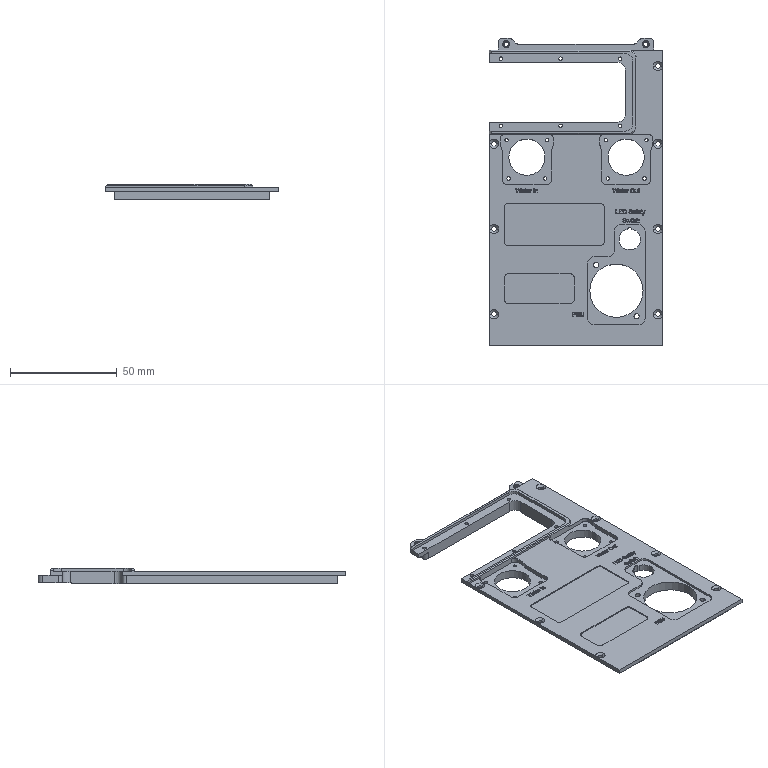NC program | NX | posted with a generic post | part box 81.5 x 144.28 x 7.5 mm
Lines 2086 to 3119 of 3119:
(CAVITY_MILL_COPY_COPY_1 , TOOL : D4精光)
N4128 T02 M6
N4130 G54
N4132 G17 G0 G90 X-24.59 Y-32.252 S6500 M3
N4134 G43 Z3.1 H2
N4136 Z-1.4
N4138 G94 G1 Z-1.9 F2000.
N4140 G3 X-24.99 Y-32.652 R0.4
N4142 G1 Y-33.3
N4144 X-24.342
N4146 G3 X-23.942 Y-32.9 R0.4
N4148 G1 Z-1.4
N4150 G0 Z0.5
N4152 X-24.59 Y-32.252
N4154 Z-1.9
N4156 G1 Z-2.4
N4158 G3 X-24.99 Y-32.652 R0.4
N4160 G1 Y-33.3
N4162 X-24.342
N4164 G3 X-23.942 Y-32.9 R0.4
N4166 G1 Z-1.9
N4168 G0 Z-1.4
N4170 X-24.59 Y-32.252
N4172 Z-2.4
N4174 G1 Z-2.9
N4176 G3 X-24.99 Y-32.652 R0.4
N4178 G1 Y-33.3
N4180 X-24.342
N4182 G3 X-23.942 Y-32.9 R0.4
N4184 G1 Z-2.4
N4186 G0 Z-1.9
N4188 X-24.59 Y-32.252
N4190 Z-2.9
N4192 G1 Z-3.4
N4194 G3 X-24.99 Y-32.652 R0.4
N4196 G1 Y-33.3
N4198 X-24.342
N4200 G3 X-23.942 Y-32.9 R0.4
N4202 G1 Z-2.9
N4204 G0 Z3.
N4206 Y-13.2
N4208 Z-1.4
N4210 G1 Z-1.9
N4212 G3 X-24.342 Y-12.8 R0.4
N4214 G1 X-24.99
N4216 Y-13.448
N4218 G3 X-24.59 Y-13.848 R0.4
N4220 G1 Z-1.4
N4222 G0 Z0.5
N4224 X-23.942 Y-13.2
N4226 Z-1.9
N4228 G1 Z-2.4
N4230 G3 X-24.342 Y-12.8 R0.4
N4232 G1 X-24.99
N4234 Y-13.448
N4236 G3 X-24.59 Y-13.848 R0.4
N4238 G1 Z-1.9
N4240 G0 Z-1.4
N4242 X-23.942 Y-13.2
N4244 Z-2.4
N4246 G1 Z-2.9
N4248 G3 X-24.342 Y-12.8 R0.4
N4250 G1 X-24.99
N4252 Y-13.448
N4254 G3 X-24.59 Y-13.848 R0.4
N4256 G1 Z-2.4
N4258 G0 Z-1.9
N4260 X-23.942 Y-13.2
N4262 Z-2.9
N4264 G1 Z-3.4
N4266 G3 X-24.342 Y-12.8 R0.4
N4268 G1 X-24.99
N4270 Y-13.448
N4272 G3 X-24.59 Y-13.848 R0.4
N4274 G1 Z-2.9
N4276 G0 Z3.
N4278 X-6.09 Y-14.648
N4280 Z-1.4
N4282 G1 Z-1.9
N4284 G3 X-5.69 Y-14.248 R0.4
N4286 G1 Y-13.6
N4288 X-6.338
N4290 G3 X-6.738 Y-14. R0.4
N4292 G1 Z-1.4
N4294 G0 Z0.5
N4296 X-6.09 Y-14.648
N4298 Z-1.9
N4300 G1 Z-2.4
N4302 G3 X-5.69 Y-14.248 R0.4
N4304 G1 Y-13.6
N4306 X-6.338
N4308 G3 X-6.738 Y-14. R0.4
N4310 G1 Z-1.9
N4312 G0 Z-1.4
N4314 X-6.09 Y-14.648
N4316 Z-2.4
N4318 G1 Z-2.9
N4320 G3 X-5.69 Y-14.248 R0.4
N4322 G1 Y-13.6
N4324 X-6.338
N4326 G3 X-6.738 Y-14. R0.4
N4328 G1 Z-2.4
N4330 G0 Z-1.9
N4332 X-6.09 Y-14.648
N4334 Z-2.9
N4336 G1 Z-3.4
N4338 G3 X-5.69 Y-14.248 R0.4
N4340 G1 Y-13.6
N4342 X-6.338
N4344 G3 X-6.738 Y-14. R0.4
N4346 G1 Z-2.9
N4348 G0 Z3.
N4350 Y-32.1
N4352 Z-1.4
N4354 G1 Z-1.9
N4356 G3 X-6.338 Y-32.5 R0.4
N4358 G1 X-5.69
N4360 Y-31.852
N4362 G3 X-6.09 Y-31.452 R0.4
N4364 G1 Z-1.4
N4366 G0 Z0.5
N4368 X-6.738 Y-32.1
N4370 Z-1.9
N4372 G1 Z-2.4
N4374 G3 X-6.338 Y-32.5 R0.4
N4376 G1 X-5.69
N4378 Y-31.852
N4380 G3 X-6.09 Y-31.452 R0.4
N4382 G1 Z-1.9
N4384 G0 Z-1.4
N4386 X-6.738 Y-32.1
N4388 Z-2.4
N4390 G1 Z-2.9
N4392 G3 X-6.338 Y-32.5 R0.4
N4394 G1 X-5.69
N4396 Y-31.852
N4398 G3 X-6.09 Y-31.452 R0.4
N4400 G1 Z-2.4
N4402 G0 Z-1.9
N4404 X-6.738 Y-32.1
N4406 Z-2.9
N4408 G1 Z-3.4
N4410 G3 X-6.338 Y-32.5 R0.4
N4412 G1 X-5.69
N4414 Y-31.852
N4416 G3 X-6.09 Y-31.452 R0.4
N4418 G1 Z-2.9
N4420 G0 Z3.
N4422 X7.81 Y-30.602
N4424 Z-1.4
N4426 G1 Z-1.9
N4428 G3 X7.41 Y-31.002 R0.4
N4430 G1 Y-31.65
N4432 X8.058
N4434 G3 X8.458 Y-31.25 R0.4
N4436 G1 Z-1.4
N4438 G0 Z3.
N4440 X22.162
N4442 Z-1.4
N4444 G1 Z-1.9
N4446 G3 X22.562 Y-31.65 R0.4
N4448 G1 X23.21
N4450 Y-31.002
N4452 G3 X22.81 Y-30.602 R0.4
N4454 G1 Z-1.4
N4456 G0 Z3.
N4458 X40.81
N4460 Z-1.4
N4462 G1 Z-1.9
N4464 G3 X40.41 Y-31.002 R0.4
N4466 G1 Y-31.65
N4468 X41.058
N4470 G3 X41.458 Y-31.25 R0.4
N4472 G1 Z-1.4
N4474 G0 Z3.
N4476 X49.162
N4478 Z-1.4
N4480 G1 Z-1.9
N4482 G3 X49.562 Y-31.65 R0.4
N4484 G1 X50.21
N4486 Y-31.002
N4488 G3 X49.81 Y-30.602 R0.4
N4490 G1 Z-1.4
N4492 G0 Z3.
N4494 Y-3.898
N4496 Z-1.4
N4498 G1 Z-1.9
N4500 G3 X50.21 Y-3.498 R0.4
N4502 G1 Y-2.85
N4504 X49.562
N4506 G3 X49.162 Y-3.25 R0.4
N4508 G1 Z-1.4
N4510 G0 Z3.
N4512 X41.458
N4514 Z-1.4
N4516 G1 Z-1.9
N4518 G3 X41.058 Y-2.85 R0.4
N4520 G1 X40.41
N4522 Y-3.498
N4524 G3 X40.81 Y-3.898 R0.4
N4526 G1 Z-1.4
N4528 G0 Z3.
N4530 X22.81 Y10.102
N4532 Z-1.4
N4534 G1 Z-1.9
N4536 G3 X23.21 Y10.502 R0.4
N4538 G1 Y11.15
N4540 X22.562
N4542 G3 X22.162 Y10.75 R0.4
N4544 G1 Z-1.4
N4546 G0 Z3.
N4548 X8.458
N4550 Z-1.4
N4552 G1 Z-1.9
N4554 G3 X8.058 Y11.15 R0.4
N4556 G1 X7.41
N4558 Y10.502
N4560 G3 X7.81 Y10.102 R0.4
N4562 G1 Z-1.4
N4564 G0 Z3.
N4566 X-6.738 Y14.5
N4568 Z-1.4
N4570 G1 Z-1.9
N4572 G3 X-6.338 Y14.1 R0.4
N4574 G1 X-5.69
N4576 Y14.748
N4578 G3 X-6.09 Y15.148 R0.4
N4580 G1 Z-1.4
N4582 G0 Z0.5
N4584 X-6.738 Y14.5
N4586 Z-1.9
N4588 G1 Z-2.4
N4590 G3 X-6.338 Y14.1 R0.4
N4592 G1 X-5.69
N4594 Y14.748
N4596 G3 X-6.09 Y15.148 R0.4
N4598 G1 Z-1.9
N4600 G0 Z-1.4
N4602 X-6.738 Y14.5
N4604 Z-2.4
N4606 G1 Z-2.9
N4608 G3 X-6.338 Y14.1 R0.4
N4610 G1 X-5.69
N4612 Y14.748
N4614 G3 X-6.09 Y15.148 R0.4
N4616 G1 Z-2.4
N4618 G0 Z-1.9
N4620 X-6.738 Y14.5
N4622 Z-2.9
N4624 G1 Z-3.4
N4626 G3 X-6.338 Y14.1 R0.4
N4628 G1 X-5.69
N4630 Y14.748
N4632 G3 X-6.09 Y15.148 R0.4
N4634 G1 Z-2.9
N4636 G0 Z3.
N4638 Y31.952
N4640 Z-1.4
N4642 G1 Z-1.9
N4644 G3 X-5.69 Y32.352 R0.4
N4646 G1 Y33.
N4648 X-6.338
N4650 G3 X-6.738 Y32.6 R0.4
N4652 G1 Z-1.4
N4654 G0 Z0.5
N4656 X-6.09 Y31.952
N4658 Z-1.9
N4660 G1 Z-2.4
N4662 G3 X-5.69 Y32.352 R0.4
N4664 G1 Y33.
N4666 X-6.338
N4668 G3 X-6.738 Y32.6 R0.4
N4670 G1 Z-1.9
N4672 G0 Z-1.4
N4674 X-6.09 Y31.952
N4676 Z-2.4
N4678 G1 Z-2.9
N4680 G3 X-5.69 Y32.352 R0.4
N4682 G1 Y33.
N4684 X-6.338
N4686 G3 X-6.738 Y32.6 R0.4
N4688 G1 Z-2.4
N4690 G0 Z-1.9
N4692 X-6.09 Y31.952
N4694 Z-2.9
N4696 G1 Z-3.4
N4698 G3 X-5.69 Y32.352 R0.4
N4700 G1 Y33.
N4702 X-6.338
N4704 G3 X-6.738 Y32.6 R0.4
N4706 G1 Z-2.9
N4708 G0 Z3.
N4710 X-23.942 Y33.4
N4712 Z-1.4
N4714 G1 Z-1.9
N4716 G3 X-24.342 Y33.8 R0.4
N4718 G1 X-24.99
N4720 Y33.152
N4722 G3 X-24.59 Y32.752 R0.4
N4724 G1 Z-1.4
N4726 G0 Z0.5
N4728 X-23.942 Y33.4
N4730 Z-1.9
N4732 G1 Z-2.4
N4734 G3 X-24.342 Y33.8 R0.4
N4736 G1 X-24.99
N4738 Y33.152
N4740 G3 X-24.59 Y32.752 R0.4
N4742 G1 Z-1.9
N4744 G0 Z-1.4
N4746 X-23.942 Y33.4
N4748 Z-2.4
N4750 G1 Z-2.9
N4752 G3 X-24.342 Y33.8 R0.4
N4754 G1 X-24.99
N4756 Y33.152
N4758 G3 X-24.59 Y32.752 R0.4
N4760 G1 Z-2.4
N4762 G0 Z-1.9
N4764 X-23.942 Y33.4
N4766 Z-2.9
N4768 G1 Z-3.4
N4770 G3 X-24.342 Y33.8 R0.4
N4772 G1 X-24.99
N4774 Y33.152
N4776 G3 X-24.59 Y32.752 R0.4
N4778 G1 Z-2.9
N4780 G0 Z3.
N4782 Y14.348
N4784 Z-1.4
N4786 G1 Z-1.9
N4788 G3 X-24.99 Y13.948 R0.4
N4790 G1 Y13.3
N4792 X-24.342
N4794 G3 X-23.942 Y13.7 R0.4
N4796 G1 Z-1.4
N4798 G0 Z0.5
N4800 X-24.59 Y14.348
N4802 Z-1.9
N4804 G1 Z-2.4
N4806 G3 X-24.99 Y13.948 R0.4
N4808 G1 Y13.3
N4810 X-24.342
N4812 G3 X-23.942 Y13.7 R0.4
N4814 G1 Z-1.9
N4816 G0 Z-1.4
N4818 X-24.59 Y14.348
N4820 Z-2.4
N4822 G1 Z-2.9
N4824 G3 X-24.99 Y13.948 R0.4
N4826 G1 Y13.3
N4828 X-24.342
N4830 G3 X-23.942 Y13.7 R0.4
N4832 G1 Z-2.4
N4834 G0 Z-1.9
N4836 X-24.59 Y14.348
N4838 Z-2.9
N4840 G1 Z-3.4
N4842 G3 X-24.99 Y13.948 R0.4
N4844 G1 Y13.3
N4846 X-24.342
N4848 G3 X-23.942 Y13.7 R0.4
N4850 G1 Z-2.9
N4852 G0 Z3.1
(FLOOR_WALL_1_COPY , TOOL : D4精光)
N4854 Z50. S5000
N4856 X15.11 Y-9.428
N4858 Z-0.5
N4860 G1 Y-23.95 Z-1.261 F700.
N4862 X15.51 Z-1.282
N4864 Y-10.25 Z-2.
N4866 Y3.45
N4868 X15.11
N4870 Y-23.95
N4872 X15.51
N4874 Y-10.25
N4876 X17.31
N4878 Y5.25
N4880 X13.31
N4882 Y-25.75
N4884 X17.31
N4886 Y-10.25
N4888 X20.31
N4890 Y8.25
N4892 X10.31
N4894 Y-28.75
N4896 X20.31
N4898 Y-10.25
N4900 X23.31
N4902 Y11.25
N4904 X7.31
N4906 Y-31.75
N4908 X23.31
N4910 Y-10.25
N4912 Y-9.25
N4914 Z-1.5
N4916 G0 Z50.
N4918 X45.51 Y-26.072
N4920 Z-0.5
N4922 G1 Y-7.55 Z-1.471
N4924 X45.11 Z-1.492
N4926 Y-17.25 Z-2.
N4928 Y-26.95
N4930 X45.51
N4932 Y-7.55
N4934 X45.11
N4936 Y-17.25
N4938 X43.31
N4940 Y-28.75
N4942 X47.31
N4944 Y-5.75
N4946 X43.31
N4948 Y-17.25
N4950 X40.31
N4952 Y-31.75
N4954 X50.31
N4956 Y-2.75
N4958 X40.31
N4960 Y-17.25
N4962 Y-18.25
N4964 Z-1.5
N4966 G0 Z50.
N4968 X42.604 Y19.179
N4970 Z-0.5
N4972 G1 X42.671 Y18.957 Z-0.512
N4974 X42.812 Y18.3 Z-0.547
N4976 X49.46 Z-0.896
N4978 Y19.6 Z-0.964
N4980 X42.476 Z-1.33
N4982 X42.671 Y18.957 Z-1.365
N4984 X42.812 Y18.3 Z-1.4
N4986 X49.46 Z-1.749
N4988 Y19.6 Z-1.817
N4990 X45.968 Z-2.
N4992 X42.476
N4994 G2 X42.812 Y18.3 R15.8
N4996 G1 X49.46
N4998 Y19.6
N5000 X45.968
N5002 Y21.4
N5004 X39.812
N5006 X38.064 Y22.392
N5008 X39.812 Y21.4
N5010 G2 X41.279 Y16.5 R14.
N5012 G1 X51.26
N5014 Y21.4
N5016 X45.968
N5018 Y24.4
N5020 X33.073
N5022 X31.077 Y24.284
N5024 G3 X27.36 Y25. R10.
N5026 G1 X22.31
N5028 Y25.4
N5030 X31.341
N5032 G3 X31.077 Y24.284 R2.
N5034 G1 X33.073 Y24.4
N5036 G2 X38.36 Y15. R11.
N5038 G1 Y13.5
N5040 X54.26
N5042 Y24.4
N5044 X45.968
N5046 Y27.4
N5048 X20.31
N5050 Y23.
N5052 X27.36
N5054 G2 X35.36 Y15. R8.
N5056 G1 Y10.5
N5058 X57.26
N5060 Y27.4
N5062 X45.968
N5064 Y30.4
N5066 X18.31
N5068 G3 X17.31 Y29.4 R1.
N5070 G1 Y21.
N5072 G3 X18.31 Y20. R1.
N5074 G1 X27.36
N5076 G2 X32.36 Y15. R5.
N5078 G1 Y8.5
N5080 G3 X33.36 Y7.5 R1.
N5082 G1 X59.26
N5084 G3 X60.26 Y8.5 R1.
N5086 G1 Y29.4
N5088 G3 X59.26 Y30.4 R1.
N5090 G1 X45.968
N5092 X44.968
N5094 Z-1.5
N5096 G0 Z50.
N5098 X48.772 Y19.6
N5100 Z-1.5
N5102 G1 X42.476 Z-1.83
N5104 X42.671 Y18.957 Z-1.865
N5106 X42.812 Y18.3 Z-1.9
N5108 X49.46 Z-2.249
N5110 Y19.6 Z-2.317
N5112 X45.968 Z-2.5
N5114 X42.476
N5116 G2 X42.812 Y18.3 R15.8
N5118 G1 X49.46
N5120 Y19.6
N5122 X45.968
N5124 Y21.4
N5126 X39.812
N5128 X38.064 Y22.392
N5130 X39.812 Y21.4
N5132 G2 X41.279 Y16.5 R14.
N5134 G1 X51.26
N5136 Y21.4
N5138 X45.968
N5140 Y24.4
N5142 X33.073
N5144 X31.077 Y24.284
N5146 G3 X27.36 Y25. R10.
N5148 G1 X22.31
N5150 Y25.4
N5152 X31.341
N5154 G3 X31.077 Y24.284 R2.
N5156 G1 X33.073 Y24.4
N5158 G2 X38.36 Y15. R11.
N5160 G1 Y13.5
N5162 X54.26
N5164 Y24.4
N5166 X45.968
N5168 Y27.4
N5170 X20.31
N5172 Y23.
N5174 X27.36
N5176 G2 X35.36 Y15. R8.
N5178 G1 Y10.5
N5180 X57.26
N5182 Y27.4
N5184 X45.968
N5186 Y30.4
N5188 X18.31
N5190 G3 X17.31 Y29.4 R1.
N5192 G1 Y21.
N5194 G3 X18.31 Y20. R1.
N5196 G1 X27.36
N5198 G2 X32.36 Y15. R5.
N5200 G1 Y8.5
N5202 G3 X33.36 Y7.5 R1.
N5204 G1 X59.26
N5206 G3 X60.26 Y8.5 R1.
N5208 G1 Y29.4
N5210 G3 X59.26 Y30.4 R1.
N5212 G1 X45.968
N5214 X44.968
N5216 Z-2.
N5218 G0 Z50.
N5220 X-15.925 Y27.1
N5222 Z-2.
N5224 G1 X-19.09 Y27.103 Z-2.166
N5226 Y19.997 Z-2.538
N5228 X-11.59 Y20. Z-2.931
N5230 Y27.1 Z-3.303
N5232 X-15.34 Z-3.5
N5234 Y24.1
N5236 X-16.09
N5238 Y23.
N5240 X-14.59
N5242 Y24.1
N5244 X-15.34
N5246 Y27.1
N5248 X-18.841
N5250 G2 X-19.09 Y27.103 R10.
N5252 G1 Y19.997
N5254 G2 X-18.841 Y20. R10.
N5256 G1 X-11.59
N5258 Y27.1
N5260 X-15.34
N5262 Y30.1
N5264 X-18.841
N5266 G2 X-20.653 Y30.339 R7.
N5268 G1 X-22.09 Y30.724
N5270 Y16.376
N5272 X-20.653 Y16.761
N5274 G2 X-18.841 Y17. R7.
N5276 G1 X-8.59
N5278 Y30.1
N5280 X-15.34
N5282 Y33.1
N5284 X-18.841
N5286 G2 X-19.876 Y33.236 R4.
N5288 G1 X-22.353 Y33.9
N5290 X-25.09
N5292 Y13.2
N5294 X-22.353
N5296 X-19.876 Y13.864
N5298 G2 X-18.841 Y14. R4.
N5300 G1 X-5.59
N5302 Y33.1
N5304 X-15.34
N5306 X-16.34
N5308 Z-3.
N5310 G0 Z50.
N5312 X-14.755 Y-26.6
N5314 Z-2.
N5316 G1 X-11.59 Z-2.166
N5318 Y-19.5 Z-2.538
N5320 X-19.09 Y-19.497 Z-2.931
N5322 Y-26.603 Z-3.303
N5324 X-15.34 Y-26.6 Z-3.5
N5326 Y-23.6
N5328 X-14.59
N5330 Y-22.5
N5332 X-16.09
N5334 Y-23.6
N5336 X-15.34
N5338 Y-26.6
N5340 X-11.59
N5342 Y-19.5
N5344 X-18.841
N5346 G2 X-19.09 Y-19.497 R10.
N5348 G1 Y-26.603
N5350 G2 X-18.841 Y-26.6 R10.
N5352 G1 X-15.34
N5354 Y-29.6
N5356 X-8.59
N5358 Y-16.5
N5360 X-18.841
N5362 G2 X-20.653 Y-16.261 R7.
N5364 G1 X-22.09 Y-15.876
N5366 Y-30.224
N5368 X-20.653 Y-29.839
N5370 G2 X-18.841 Y-29.6 R7.
N5372 G1 X-15.34
N5374 Y-32.6
N5376 X-5.59
N5378 Y-13.5
N5380 X-18.841
N5382 G2 X-19.876 Y-13.364 R4.
N5384 G1 X-22.353 Y-12.7
N5386 X-25.09
N5388 Y-33.4
N5390 X-22.353
N5392 X-19.876 Y-32.736
N5394 G2 X-18.841 Y-32.6 R4.
N5396 G1 X-15.34
N5398 X-14.34
N5400 Z-3.
N5402 G0 Z50.
N5404 M5
(HOLE_MILLING , TOOL : D2精光)
N5406 T10 M6
N5408 G54
N5410 G17 G0 G90 X-69.36 Y-32.75 S4500 M3
N5412 G43 Z50. H10
N5414 Z-3.
N5416 G94 G3 X-69.11 Y-32.5 R0.25 F300.
N5418 X-69.36 Y-32.25 R0.25
N5420 X-69.36 Y-32.25 Z-3.2 I0. J-0.5
N5422 X-69.36 Y-32.25 Z-3.4 I0. J-0.5
N5424 X-69.36 Y-32.25 Z-3.6 I0. J-0.5
N5426 X-69.36 Y-32.25 Z-3.8 I0. J-0.5
N5428 X-69.36 Y-32.25 Z-4. I0. J-0.5
N5430 X-69.36 Y-32.25 Z-4.2 I0. J-0.5
N5432 X-69.36 Y-32.25 Z-4.4 I0. J-0.5
N5434 X-69.36 Y-32.25 Z-4.6 I0. J-0.5
N5436 X-69.86 Y-32.75 R0.5
N5438 X-69.36 Y-32.25 R-0.5
N5440 X-69.61 Y-32.5 R0.25
N5442 X-69.36 Y-32.75 R0.25
N5444 G0 Z50.
N5446 Y32.75
N5448 Z-3.
N5450 G3 X-69.11 Y33. R0.25
N5452 X-69.36 Y33.25 R0.25
N5454 X-69.36 Y33.25 Z-3.2 I0. J-0.5
N5456 X-69.36 Y33.25 Z-3.4 I0. J-0.5
N5458 X-69.36 Y33.25 Z-3.6 I0. J-0.5
N5460 X-69.36 Y33.25 Z-3.8 I0. J-0.5
N5462 X-69.36 Y33.25 Z-4. I0. J-0.5
N5464 X-69.36 Y33.25 Z-4.2 I0. J-0.5
N5466 X-69.36 Y33.25 Z-4.4 I0. J-0.5
N5468 X-69.36 Y33.25 Z-4.6 I0. J-0.5
N5470 X-69.86 Y32.75 R0.5
N5472 X-69.36 Y33.25 R-0.5
N5474 X-69.61 Y33. R0.25
N5476 X-69.36 Y32.75 R0.25
N5478 G0 Z50.
N5480 M5
(DRILLING_1 , TOOL : SD-6.)
N5482 T13 M6
N5484 G54
N5486 G17 G0 G90 X-59.09 Y38.5 S2000 M3
N5488 G43 Z50. H13
N5490 G94 G81 G98 Z-3.5 F150. R1.5
N5492 X-22.61
N5494 X17.39
N5496 X57.39
N5498 Y-38.5
N5500 X17.39
N5502 X-22.61
N5504 G80
N5506 G0 X-22.61 Y-38.5 Z50.
(DRILLING_1_COPY , TOOL : SD-6.)
N5508 X-69.36 Y32.75
N5510 G81 Z-5.3 F150. R-0.5
N5512 Y-32.75
N5514 G80
N5516 G0 X-69.36 Y-32.75 Z50.
(DRILLING_1_COPY_COPY , TOOL : SD-6.)
N5518 X34.31 Y9.45
N5520 G81 Z-4.1 F150. R0.5
N5522 X58.31 Y28.45
N5524 G80
N5526 G0 X58.31 Y28.45 Z50.
(PLANAR_MILL_2_COPY_1 , TOOL : SD-6.)
N5528 X-21.09 Y-41.85 S6500
N5530 Z3.
N5532 Z0.5
N5534 G1 Z-2.5 F800.
N5536 X-27.09
N5538 X-28.59
N5540 X-34.59
N5542 Z0.5
N5544 G0 Z3.
N5546 X-21.09 Y-41.75
N5548 Z0.5
N5550 G1 Z-2.5
N5552 X-27.09
N5554 X-28.59
N5556 X-34.59
N5558 Z0.5
N5560 G0 Z3.
N5562 X-59.09 Y-41.85
N5564 Z0.5
N5566 G1 Z-2.5
N5568 X-65.09
N5570 X-66.59
N5572 X-72.59
N5574 Z0.5
N5576 G0 Z3.
N5578 X-59.09 Y-41.75
N5580 Z0.5
N5582 G1 Z-2.5
N5584 X-65.09
N5586 X-66.59
N5588 X-72.59
N5590 Z0.5
N5592 G0 Z3.
N5594 M5
(DRILLING_1_COPY_1 , TOOL : 倒角-3.)
N5596 T03 M6
N5598 G54
N5600 G17 G0 G90 X-6.34 Y14.95 S2000 M3
N5602 G43 Z10. H3
N5604 G94 G81 G98 Z-4.5 F150. R-0.5
N5606 Y32.15
N5608 X-24.34 Y33.05
N5610 X-31.102 Y20.75 Z-2.5 R1.5
N5612 X-24.34 Y14.05 Z-4.5 R-0.5
N5614 X-31.102 Y-7.25 Z-2.5 R1.5
N5616 X-24.34 Y-13.55 Z-4.5 R-0.5
N5618 X-6.34 Y-14.45
N5620 Y-31.65
N5622 X-24.34 Y-32.55
N5624 X-31.102 Y-35.25 Z-2.5 R1.5
N5626 X-62.602
N5628 Y-7.25
N5630 Y20.75
N5632 G80
N5634 G0 X-62.602 Y20.75 Z10.
(PLANAR_MILL_2 , TOOL : 倒角-3.)
N5636 Z50. S6500
N5638 X-28.84 Y-42.75
N5640 Z-0.5
N5642 G1 Z-2.5 F1500.
N5644 G3 X-29.84 Y-41.75 R1.
N5646 G1 X-32.84
N5648 G2 X-33.84 Y-40.75 R1.
N5650 G1 Y19.5
N5652 G3 X-36.59 Y22.25 R2.75
N5654 G1 X-57.09
N5656 G3 X-59.84 Y19.5 R2.75
N5658 G1 Y-40.75
N5660 G2 X-60.84 Y-41.75 R1.
N5662 G1 X-63.34
N5664 G3 X-64.34 Y-42.75 R1.
N5666 G1 Z-0.5
N5668 G0 Z50.
(PLANAR_MILL_2_COPY , TOOL : 倒角-3.)
N5670 X-23.89 Y13.1
N5672 Z1.1
N5674 G1 Z-1.9
N5676 X-25.39 Y11.628
N5678 G3 X-25.09 Y11.6 R1.6
N5680 G1 X-22.353
N5682 G3 X-21.939 Y11.655 R1.6
N5684 G1 X-19.462 Y12.318
N5686 G2 X-18.841 Y12.4 R2.4
N5688 G1 X-5.59
N5690 G3 X-3.99 Y14. R1.6
N5692 G1 Y33.1
N5694 G3 X-5.59 Y34.7 R1.6
N5696 G1 X-18.841
N5698 G2 X-19.462 Y34.782 R2.4
N5700 G1 X-21.939 Y35.445
N5702 G3 X-22.353 Y35.5 R1.6
N5704 G1 X-25.09
N5706 G3 X-26.69 Y33.9 R1.6
N5708 G1 Y28.174
N5710 X-25.19 Y28.677
N5712 Z1.1
N5714 G0 Z50.
N5716 X-23.89 Y-33.5
N5718 Z1.1
N5720 G1 Z-1.9
N5722 X-25.39 Y-34.972
N5724 G3 X-25.09 Y-35. R1.6
N5726 G1 X-22.353
N5728 G3 X-21.939 Y-34.945 R1.6
N5730 G1 X-19.462 Y-34.282
N5732 G2 X-18.841 Y-34.2 R2.4
N5734 G1 X-5.59
N5736 G3 X-3.99 Y-32.6 R1.6
N5738 G1 Y-13.5
N5740 G3 X-5.59 Y-11.9 R1.6
N5742 G1 X-18.841
N5744 G2 X-19.462 Y-11.818 R2.4
N5746 G1 X-21.939 Y-11.155
N5748 G3 X-22.353 Y-11.1 R1.6
N5750 G1 X-25.09
N5752 G3 X-25.39 Y-11.128 R1.6
N5754 G1 X-23.89 Y-12.6
N5756 Z1.1
N5758 G0 Z50.
N5760 X7.21 Y-10.25
N5762 Z1.1
N5764 G1 Z-1.9
N5766 X5.71
N5768 Y-31.75
N5770 G3 X7.31 Y-33.35 R1.6
N5772 G1 X23.31
N5774 G3 X24.91 Y-31.75 R1.6
N5776 G1 Y11.25
N5778 G3 X23.31 Y12.85 R1.6
N5780 G1 X7.31
N5782 G3 X5.71 Y11.25 R1.6
N5784 G1 Y-10.25
N5786 X7.21
N5788 Z1.1
N5790 G0 Z50.
N5792 X50.41 Y-17.25
N5794 Z1.1
N5796 G1 Z-1.9
N5798 X51.91
N5800 Y-2.75
N5802 G3 X50.31 Y-1.15 R1.6
N5804 G1 X40.31
N5806 G3 X38.71 Y-2.75 R1.6
N5808 G1 Y-31.75
N5810 G3 X40.31 Y-33.35 R1.6
N5812 G1 X50.31
N5814 G3 X51.91 Y-31.75 R1.6
N5816 G1 Y-17.25
N5818 X50.41
N5820 Z1.1
N5822 G0 Z50.
N5824 X38.785 Y30.5
N5826 Z1.1
N5828 G1 Z-1.9
N5830 Y32.
N5832 X18.31
N5834 G3 X15.71 Y29.4 R2.6
N5836 G1 Y21.
N5838 G3 X18.31 Y18.4 R2.6
N5840 G1 X27.36
N5842 G2 X30.76 Y15. R3.4
N5844 G1 Y8.5
N5846 G3 X33.36 Y5.9 R2.6
N5848 G1 X59.26
N5850 G3 X61.86 Y8.5 R2.6
N5852 G1 Y29.4
N5854 G3 X59.26 Y32. R2.6
N5856 G1 X38.785
N5858 Y30.5
N5860 Z1.1
N5862 G0 Z50.
(PLANAR_MILL_2_COPY_COPY , TOOL : 倒角-3.)
N5864 X-16.34 Y17.55
N5866 Z-1.5
N5868 G1 Z-4.5
N5870 Y16.05
N5872 G3 X-8.84 Y23.55 R7.5
N5874 X-16.34 Y16.05 R-7.5
N5876 G1 Y17.55
N5878 Z-1.5
N5880 G0 Z50.
N5882 Y-29.05
N5884 Z-1.5
N5886 G1 Z-4.5
N5888 Y-30.55
N5890 G3 X-8.84 Y-23.05 R7.5
N5892 X-16.34 Y-30.55 R-7.5
N5894 G1 Y-29.05
N5896 Z-1.5
N5898 G0 Z50.
(PLANAR_MILL_2_COPY_COPY_COPY_1 , TOOL : 倒角-3.)
N5900 X24.459 Y25.2
N5902 Z-0.5
N5904 G1 Z-3.5
N5906 X25.959
N5908 Y26.838
N5910 G3 X18.659 Y26.834 R4.
N5912 G1 Y26.2
N5914 G2 X17.659 Y25.2 R1.
N5916 X18.659 Y24.2 R1.
N5918 G1 Y23.566
N5920 G3 X25.959 Y23.562 R4.
N5922 G1 Y25.2
N5924 X24.459
N5926 Z-0.5
N5928 G0 Z50.
N5930 X46.31 Y28.95
N5932 Z-0.5
N5934 G1 Z-3.5
N5936 Y30.45
N5938 G3 X34.81 Y18.95 R11.5
N5940 X46.31 Y30.45 R-11.5
N5942 G1 Y28.95
N5944 Z-0.5
N5946 G0 Z50.
(PLANAR_MILL_2_COPY_COPY_COPY , TOOL : 倒角-3.)
N5948 X-69.09 Y27.873
N5950 Z0.5
N5952 G1 Z-2.5
N5954 X-67.59 Y27.489
N5956 Y40.75
N5958 G2 X-66.59 Y41.75 R1.
N5960 G1 X72.14
N5962 G2 X73.14 Y40.75 R1.
N5964 G1 Y-40.75
N5966 G2 X72.14 Y-41.75 R1.
N5968 G1 X-23.86
N5970 X-25.36
N5972 Y-43.25
N5974 Z0.5
N5976 G0 Z50.
(PLANAR_MILL_2_COPY_COPY_COPY_COPY , TOOL : 倒角-3.)
N5978 X-67.29 Y-42.374
N5980 Z1.8
N5982 G1 Z-1.2
N5984 Y-39.674
N5986 Y24.55
N5988 G2 X-62.59 Y29.25 R4.7
N5990 G1 X-31.09
N5992 G2 X-26.39 Y24.55 R4.7
N5994 G1 Y-39.674
N5996 Y-42.374
N5998 Z1.8
N6000 G0 Z50.
(PLANAR_MILL_2_COPY_COPY_COPY_COPY_COPY_1 , TOOL : 倒角-3.)
N6002 X-29.79
N6004 Z1.8
N6006 G1 Z-1.2
N6008 Y-39.674
N6010 Y23.
N6012 G3 X-32.34 Y25.55 R2.55
N6014 G1 X-61.34
N6016 G3 X-63.89 Y23. R2.55
N6018 G1 Y-39.674
N6020 Y-42.374
N6022 Z1.8
N6024 G0 Z50.
(PLANAR_MILL_2_COPY_COPY_COPY_COPY_COPY , TOOL : 倒角-3.)
N6026 X-69.776 Y-38.
N6028 Z-1.
N6030 G1 Z-4.
N6032 X-70.14 Y-37.
N6034 G2 X-72.64 Y-34.5 R2.5
N6036 G1 Y-31.328
N6038 G2 X-71.908 Y-29.561 R2.5
N6040 G1 X-70.279 Y-27.932
N6042 G3 X-69.84 Y-26.872 R1.5
N6044 G1 Y26.872
N6046 G3 X-70.279 Y27.932 R1.5
N6048 G1 X-71.908 Y29.561
N6050 G2 X-72.64 Y31.328 R2.5
N6052 G1 Y34.5
N6054 G2 X-70.14 Y37. R2.5
N6056 G1 X-69.776 Y38.
N6058 Z-1.
N6060 G0 Z50.
N6062 M5
(DRILLING_1_COPY_2 , TOOL : D2.4钻头)
N6064 T15 M6
N6066 G54
N6068 G17 G0 G90 X-59.09 Y38.5 S2000 M3
N6070 G43 Z50. H15
N6072 G94 G81 G98 Z-7.5 F150. R1.5
N6074 X-22.61
N6076 X17.39
N6078 X57.39
N6080 Y-38.5
N6082 X17.39
N6084 X-22.61
N6086 G80
N6088 G0 X-22.61 Y-38.5 Z50.
N6090 M5
N6092 M2